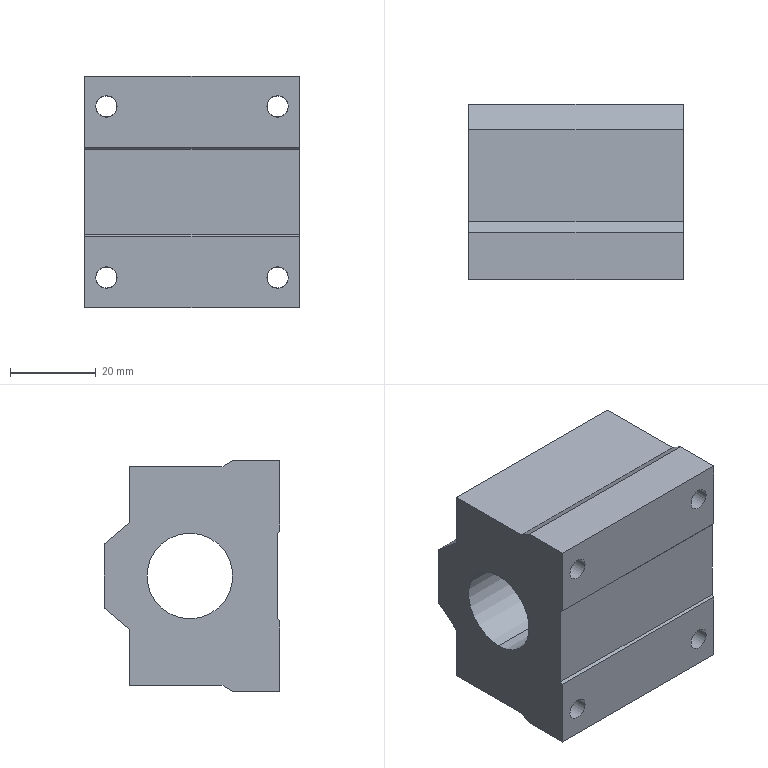Part | STEP file | Linear bearing LHBB-20 | 1 solid | 44 faces | box 50 x 41 x 54 mm | volume 78183 mm3 | cylinder 18 | plane 18 | cone 8 | commonest cylinder face diameters 4.9 x8 5 x8 20 x2